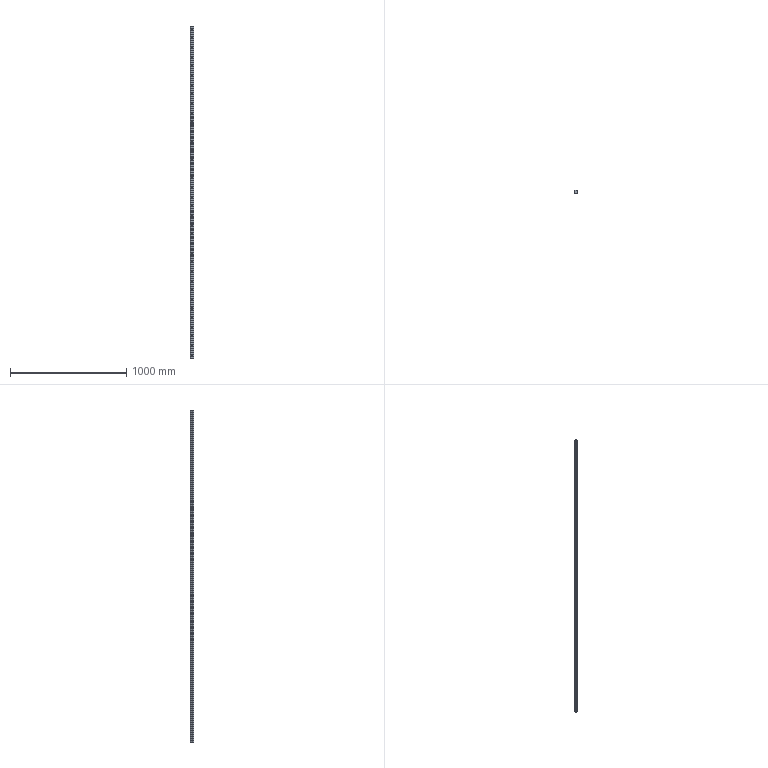Part | SolidWorks | features ICE 2, BaseBody 1, HoleWzd 1 | 1 solid | 232 faces | box 28 x 26 x 2850 mm | volume 1658147 mm3 | cylinder 166 | plane 66 | commonest cylinder face diameters 9 x72 14 x72 1.2 x12 1.6 x6 5.66 x4